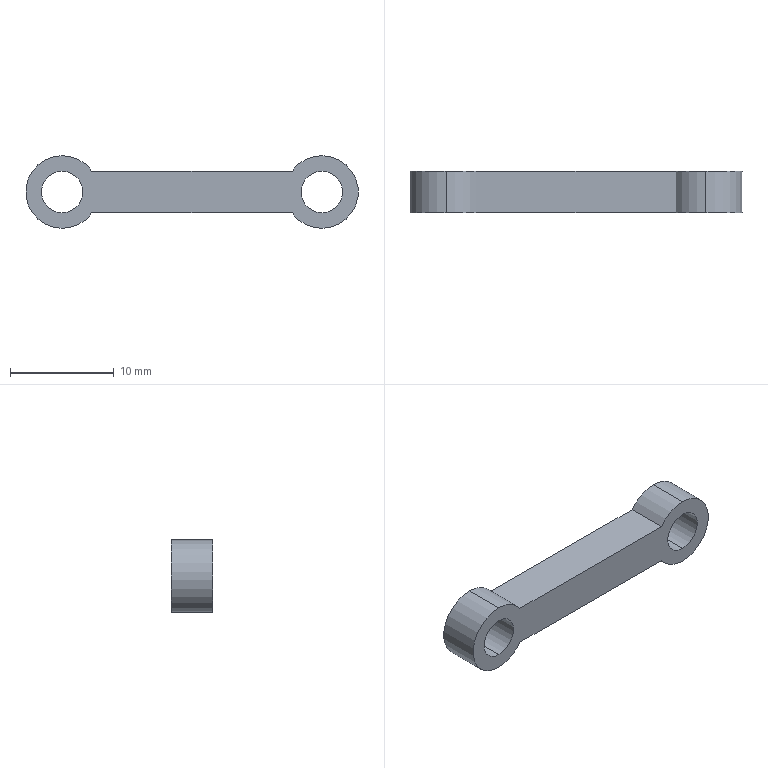Part | SolidWorks | features Extrusion 1, Scale 1 | 1 solid | 14 faces | box 32 x 4 x 7 mm | volume 501.781 mm3 | cylinder 10 | plane 4 | commonest cylinder face diameters 7 x6 4 x4
STEP:
#1=CARTESIAN_POINT('',(25.,4.,-2.));
#2=VERTEX_POINT('',#1);
#3=CARTESIAN_POINT('',(25.,4.,2.));
#4=VERTEX_POINT('',#3);
#5=CARTESIAN_POINT('',(25.,4.,0.));
#6=DIRECTION('',(0.,1.,0.));
#7=DIRECTION('',(0.,0.,1.));
#8=AXIS2_PLACEMENT_3D('',#5,#6,#7);
#9=CIRCLE('',#8,2.);
#10=EDGE_CURVE('',#2,#4,#9,.T.);
#11=ORIENTED_EDGE('',*,*,#10,.T.);
#12=CARTESIAN_POINT('',(25.,0.,2.));
#13=VERTEX_POINT('',#12);
#14=CARTESIAN_POINT('',(25.,4.,2.));
#15=DIRECTION('',(0.,-1.,0.));
#16=VECTOR('',#15,1000.);
#17=LINE('',#14,#16);
#18=EDGE_CURVE('',#4,#13,#17,.T.);
#19=ORIENTED_EDGE('',*,*,#18,.T.);
#20=CARTESIAN_POINT('',(25.,0.,-2.));
#21=VERTEX_POINT('',#20);
#22=CARTESIAN_POINT('',(25.,0.,0.));
#23=DIRECTION('',(0.,1.,0.));
#24=DIRECTION('',(0.,0.,1.));
#25=AXIS2_PLACEMENT_3D('',#22,#23,#24);
#26=CIRCLE('',#25,2.);
#27=EDGE_CURVE('',#21,#13,#26,.T.);
#28=ORIENTED_EDGE('',*,*,#27,.F.);
#29=CARTESIAN_POINT('',(25.,4.,-2.));
#30=DIRECTION('',(0.,-1.,0.));
#31=VECTOR('',#30,1000.);
#32=LINE('',#29,#31);
#33=EDGE_CURVE('',#2,#21,#32,.T.);
#34=ORIENTED_EDGE('',*,*,#33,.F.);
#35=EDGE_LOOP('',(#11,#19,#28,#34));
#36=FACE_OUTER_BOUND('',#35,.T.);
#37=CARTESIAN_POINT('',(25.,4.,0.));
#38=DIRECTION('',(0.,-1.,0.));
#39=DIRECTION('',(0.,0.,-1.));
#40=AXIS2_PLACEMENT_3D('',#37,#38,#39);
#41=CYLINDRICAL_SURFACE('',#40,2.);
#42=ADVANCED_FACE('',(#36),#41,.F.);
#43=CARTESIAN_POINT('',(0.,4.,-2.));
#44=VERTEX_POINT('',#43);
#45=CARTESIAN_POINT('',(0.,4.,2.));
#46=VERTEX_POINT('',#45);
#47=CARTESIAN_POINT('',(0.,4.,0.));
#48=DIRECTION('',(0.,1.,0.));
#49=DIRECTION('',(0.,0.,1.));
#50=AXIS2_PLACEMENT_3D('',#47,#48,#49);
#51=CIRCLE('',#50,2.);
#52=EDGE_CURVE('',#44,#46,#51,.T.);
#53=ORIENTED_EDGE('',*,*,#52,.T.);
#54=CARTESIAN_POINT('',(0.,0.,2.));
#55=VERTEX_POINT('',#54);
#56=CARTESIAN_POINT('',(0.,4.,2.));
#57=DIRECTION('',(0.,-1.,0.));
#58=VECTOR('',#57,1000.);
#59=LINE('',#56,#58);
#60=EDGE_CURVE('',#46,#55,#59,.T.);
#61=ORIENTED_EDGE('',*,*,#60,.T.);
#62=CARTESIAN_POINT('',(0.,0.,-2.));
#63=VERTEX_POINT('',#62);
#64=CARTESIAN_POINT('',(0.,0.,0.));
#65=DIRECTION('',(0.,1.,0.));
#66=DIRECTION('',(0.,0.,1.));
#67=AXIS2_PLACEMENT_3D('',#64,#65,#66);
#68=CIRCLE('',#67,2.);
#69=EDGE_CURVE('',#63,#55,#68,.T.);
#70=ORIENTED_EDGE('',*,*,#69,.F.);
#71=CARTESIAN_POINT('',(0.,4.,-2.));
#72=DIRECTION('',(0.,-1.,0.));
#73=VECTOR('',#72,1000.);
#74=LINE('',#71,#73);
#75=EDGE_CURVE('',#44,#63,#74,.T.);
#76=ORIENTED_EDGE('',*,*,#75,.F.);
#77=EDGE_LOOP('',(#53,#61,#70,#76));
#78=FACE_OUTER_BOUND('',#77,.T.);
#79=CARTESIAN_POINT('',(0.,4.,0.));
#80=DIRECTION('',(0.,-1.,0.));
#81=DIRECTION('',(0.,0.,-1.));
#82=AXIS2_PLACEMENT_3D('',#79,#80,#81);
#83=CYLINDRICAL_SURFACE('',#82,2.);
#84=ADVANCED_FACE('',(#78),#83,.F.);
#85=CARTESIAN_POINT('',(25.,4.,3.5));
#86=VERTEX_POINT('',#85);
#87=CARTESIAN_POINT('',(25.,4.,-3.5));
#88=VERTEX_POINT('',#87);
#89=CARTESIAN_POINT('',(25.,4.,0.));
#90=DIRECTION('',(0.,1.,0.));
#91=DIRECTION('',(0.,0.,1.));
#92=AXIS2_PLACEMENT_3D('',#89,#90,#91);
#93=CIRCLE('',#92,3.5);
#94=EDGE_CURVE('',#86,#88,#93,.T.);
#95=ORIENTED_EDGE('',*,*,#94,.F.);
#96=CARTESIAN_POINT('',(25.,0.,3.5));
#97=VERTEX_POINT('',#96);
#98=CARTESIAN_POINT('',(25.,4.,3.5));
#99=DIRECTION('',(0.,-1.,0.));
#100=VECTOR('',#99,1000.);
#101=LINE('',#98,#100);
#102=EDGE_CURVE('',#86,#97,#101,.T.);
#103=ORIENTED_EDGE('',*,*,#102,.T.);
#104=CARTESIAN_POINT('',(25.,0.,-3.5));
#105=VERTEX_POINT('',#104);
#106=CARTESIAN_POINT('',(25.,0.,0.));
#107=DIRECTION('',(0.,1.,0.));
#108=DIRECTION('',(0.,0.,1.));
#109=AXIS2_PLACEMENT_3D('',#106,#107,#108);
#110=CIRCLE('',#109,3.5);
#111=EDGE_CURVE('',#97,#105,#110,.T.);
#112=ORIENTED_EDGE('',*,*,#111,.T.);
#113=CARTESIAN_POINT('',(25.,4.,-3.5));
#114=DIRECTION('',(0.,-1.,0.));
#115=VECTOR('',#114,1000.);
#116=LINE('',#113,#115);
#117=EDGE_CURVE('',#88,#105,#116,.T.);
#118=ORIENTED_EDGE('',*,*,#117,.F.);
#119=EDGE_LOOP('',(#95,#103,#112,#118));
#120=FACE_OUTER_BOUND('',#119,.T.);
#121=CARTESIAN_POINT('',(25.,4.,0.));
#122=DIRECTION('',(0.,-1.,0.));
#123=DIRECTION('',(0.,0.,-1.));
#124=AXIS2_PLACEMENT_3D('',#121,#122,#123);
#125=CYLINDRICAL_SURFACE('',#124,3.5);
#126=ADVANCED_FACE('',(#120),#125,.T.);
#127=CARTESIAN_POINT('',(22.128,4.,-2.));
#128=VERTEX_POINT('',#127);
#129=CARTESIAN_POINT('',(25.,4.,0.));
#130=DIRECTION('',(0.,1.,0.));
#131=DIRECTION('',(0.,0.,1.));
#132=AXIS2_PLACEMENT_3D('',#129,#130,#131);
#133=CIRCLE('',#132,3.5);
#134=EDGE_CURVE('',#88,#128,#133,.T.);
#135=ORIENTED_EDGE('',*,*,#134,.F.);
#136=ORIENTED_EDGE('',*,*,#117,.T.);
#137=CARTESIAN_POINT('',(22.128,0.,-2.));
#138=VERTEX_POINT('',#137);
#139=CARTESIAN_POINT('',(25.,0.,0.));
#140=DIRECTION('',(0.,1.,0.));
#141=DIRECTION('',(0.,0.,1.));
#142=AXIS2_PLACEMENT_3D('',#139,#140,#141);
#143=CIRCLE('',#142,3.5);
#144=EDGE_CURVE('',#105,#138,#143,.T.);
#145=ORIENTED_EDGE('',*,*,#144,.T.);
#146=CARTESIAN_POINT('',(22.128,4.,-2.));
#147=DIRECTION('',(0.,-1.,0.));
#148=VECTOR('',#147,1000.);
#149=LINE('',#146,#148);
#150=EDGE_CURVE('',#128,#138,#149,.T.);
#151=ORIENTED_EDGE('',*,*,#150,.F.);
#152=EDGE_LOOP('',(#135,#136,#145,#151));
#153=FACE_OUTER_BOUND('',#152,.T.);
#154=CARTESIAN_POINT('',(25.,4.,0.));
#155=DIRECTION('',(0.,-1.,0.));
#156=DIRECTION('',(0.,0.,-1.));
#157=AXIS2_PLACEMENT_3D('',#154,#155,#156);
#158=CYLINDRICAL_SURFACE('',#157,3.5);
#159=ADVANCED_FACE('',(#153),#158,.T.);
#160=CARTESIAN_POINT('',(0.,4.,3.5));
#161=VERTEX_POINT('',#160);
#162=CARTESIAN_POINT('',(2.872,4.,2.));
#163=VERTEX_POINT('',#162);
#164=CARTESIAN_POINT('',(0.,4.,0.));
#165=DIRECTION('',(0.,1.,0.));
#166=DIRECTION('',(0.,0.,1.));
#167=AXIS2_PLACEMENT_3D('',#164,#165,#166);
#168=CIRCLE('',#167,3.5);
#169=EDGE_CURVE('',#161,#163,#168,.T.);
#170=ORIENTED_EDGE('',*,*,#169,.F.);
#171=CARTESIAN_POINT('',(0.,0.,3.5));
#172=VERTEX_POINT('',#171);
#173=CARTESIAN_POINT('',(0.,4.,3.5));
#174=DIRECTION('',(0.,-1.,0.));
#175=VECTOR('',#174,1000.);
#176=LINE('',#173,#175);
#177=EDGE_CURVE('',#161,#172,#176,.T.);
#178=ORIENTED_EDGE('',*,*,#177,.T.);
#179=CARTESIAN_POINT('',(2.872,0.,2.));
#180=VERTEX_POINT('',#179);
#181=CARTESIAN_POINT('',(0.,0.,0.));
#182=DIRECTION('',(0.,1.,0.));
#183=DIRECTION('',(0.,0.,1.));
#184=AXIS2_PLACEMENT_3D('',#181,#182,#183);
#185=CIRCLE('',#184,3.5);
#186=EDGE_CURVE('',#172,#180,#185,.T.);
#187=ORIENTED_EDGE('',*,*,#186,.T.);
#188=CARTESIAN_POINT('',(2.872,4.,2.));
#189=DIRECTION('',(0.,-1.,0.));
#190=VECTOR('',#189,1000.);
#191=LINE('',#188,#190);
#192=EDGE_CURVE('',#163,#180,#191,.T.);
#193=ORIENTED_EDGE('',*,*,#192,.F.);
#194=EDGE_LOOP('',(#170,#178,#187,#193));
#195=FACE_OUTER_BOUND('',#194,.T.);
#196=CARTESIAN_POINT('',(0.,4.,0.));
#197=DIRECTION('',(0.,-1.,0.));
#198=DIRECTION('',(0.,0.,-1.));
#199=AXIS2_PLACEMENT_3D('',#196,#197,#198);
#200=CYLINDRICAL_SURFACE('',#199,3.5);
#201=ADVANCED_FACE('',(#195),#200,.T.);
#202=ORIENTED_EDGE('',*,*,#177,.F.);
#203=CARTESIAN_POINT('',(0.,4.,-3.5));
#204=VERTEX_POINT('',#203);
#205=CARTESIAN_POINT('',(0.,4.,0.));
#206=DIRECTION('',(0.,1.,0.));
#207=DIRECTION('',(0.,0.,1.));
#208=AXIS2_PLACEMENT_3D('',#205,#206,#207);
#209=CIRCLE('',#208,3.5);
#210=EDGE_CURVE('',#204,#161,#209,.T.);
#211=ORIENTED_EDGE('',*,*,#210,.F.);
#212=CARTESIAN_POINT('',(0.,0.,-3.5));
#213=VERTEX_POINT('',#212);
#214=CARTESIAN_POINT('',(0.,4.,-3.5));
#215=DIRECTION('',(0.,-1.,0.));
#216=VECTOR('',#215,1000.);
#217=LINE('',#214,#216);
#218=EDGE_CURVE('',#204,#213,#217,.T.);
#219=ORIENTED_EDGE('',*,*,#218,.T.);
#220=CARTESIAN_POINT('',(0.,0.,0.));
#221=DIRECTION('',(0.,1.,0.));
#222=DIRECTION('',(0.,0.,1.));
#223=AXIS2_PLACEMENT_3D('',#220,#221,#222);
#224=CIRCLE('',#223,3.5);
#225=EDGE_CURVE('',#213,#172,#224,.T.);
#226=ORIENTED_EDGE('',*,*,#225,.T.);
#227=EDGE_LOOP('',(#202,#211,#219,#226));
#228=FACE_OUTER_BOUND('',#227,.T.);
#229=CARTESIAN_POINT('',(0.,4.,0.));
#230=DIRECTION('',(0.,-1.,0.));
#231=DIRECTION('',(0.,0.,-1.));
#232=AXIS2_PLACEMENT_3D('',#229,#230,#231);
#233=CYLINDRICAL_SURFACE('',#232,3.5);
#234=ADVANCED_FACE('',(#228),#233,.T.);
#235=ORIENTED_EDGE('',*,*,#52,.F.);
#236=CARTESIAN_POINT('',(0.,4.,0.));
#237=DIRECTION('',(0.,1.,0.));
#238=DIRECTION('',(0.,0.,1.));
#239=AXIS2_PLACEMENT_3D('',#236,#237,#238);
#240=CIRCLE('',#239,2.);
#241=EDGE_CURVE('',#46,#44,#240,.T.);
#242=ORIENTED_EDGE('',*,*,#241,.F.);
#243=EDGE_LOOP('',(#235,#242));
#244=FACE_BOUND('',#243,.T.);
#245=CARTESIAN_POINT('',(2.872,4.,-2.));
#246=VERTEX_POINT('',#245);
#247=CARTESIAN_POINT('',(0.,4.,0.));
#248=DIRECTION('',(0.,1.,0.));
#249=DIRECTION('',(0.,0.,1.));
#250=AXIS2_PLACEMENT_3D('',#247,#248,#249);
#251=CIRCLE('',#250,3.5);
#252=EDGE_CURVE('',#246,#204,#251,.T.);
#253=ORIENTED_EDGE('',*,*,#252,.T.);
#254=ORIENTED_EDGE('',*,*,#210,.T.);
#255=ORIENTED_EDGE('',*,*,#169,.T.);
#256=CARTESIAN_POINT('',(22.128,4.,2.));
#257=VERTEX_POINT('',#256);
#258=CARTESIAN_POINT('',(2.872,4.,2.));
#259=DIRECTION('',(1.,0.,0.));
#260=VECTOR('',#259,1000.);
#261=LINE('',#258,#260);
#262=EDGE_CURVE('',#163,#257,#261,.T.);
#263=ORIENTED_EDGE('',*,*,#262,.T.);
#264=CARTESIAN_POINT('',(25.,4.,0.));
#265=DIRECTION('',(0.,1.,0.));
#266=DIRECTION('',(0.,0.,1.));
#267=AXIS2_PLACEMENT_3D('',#264,#265,#266);
#268=CIRCLE('',#267,3.5);
#269=EDGE_CURVE('',#257,#86,#268,.T.);
#270=ORIENTED_EDGE('',*,*,#269,.T.);
#271=ORIENTED_EDGE('',*,*,#94,.T.);
#272=ORIENTED_EDGE('',*,*,#134,.T.);
#273=CARTESIAN_POINT('',(2.872,4.,-2.));
#274=DIRECTION('',(-1.,0.,0.));
#275=VECTOR('',#274,1000.);
#276=LINE('',#273,#275);
#277=EDGE_CURVE('',#128,#246,#276,.T.);
#278=ORIENTED_EDGE('',*,*,#277,.T.);
#279=EDGE_LOOP('',(#253,#254,#255,#263,#270,#271,#272,#278));
#280=FACE_OUTER_BOUND('',#279,.T.);
#281=ORIENTED_EDGE('',*,*,#10,.F.);
#282=CARTESIAN_POINT('',(25.,4.,0.));
#283=DIRECTION('',(0.,1.,0.));
#284=DIRECTION('',(0.,0.,1.));
#285=AXIS2_PLACEMENT_3D('',#282,#283,#284);
#286=CIRCLE('',#285,2.);
#287=EDGE_CURVE('',#4,#2,#286,.T.);
#288=ORIENTED_EDGE('',*,*,#287,.F.);
#289=EDGE_LOOP('',(#281,#288));
#290=FACE_BOUND('',#289,.T.);
#291=CARTESIAN_POINT('',(0.,4.,0.));
#292=DIRECTION('',(0.,1.,0.));
#293=DIRECTION('',(0.,0.,1.));
#294=AXIS2_PLACEMENT_3D('',#291,#292,#293);
#295=PLANE('',#294);
#296=ADVANCED_FACE('',(#244,#280,#290),#295,.T.);
#297=CARTESIAN_POINT('',(2.872,0.,-2.));
#298=VERTEX_POINT('',#297);
#299=CARTESIAN_POINT('',(0.,0.,0.));
#300=DIRECTION('',(0.,1.,0.));
#301=DIRECTION('',(0.,0.,1.));
#302=AXIS2_PLACEMENT_3D('',#299,#300,#301);
#303=CIRCLE('',#302,3.5);
#304=EDGE_CURVE('',#298,#213,#303,.T.);
#305=ORIENTED_EDGE('',*,*,#304,.F.);
#306=CARTESIAN_POINT('',(2.872,0.,-2.));
#307=DIRECTION('',(-1.,0.,0.));
#308=VECTOR('',#307,1000.);
#309=LINE('',#306,#308);
#310=EDGE_CURVE('',#138,#298,#309,.T.);
#311=ORIENTED_EDGE('',*,*,#310,.F.);
#312=ORIENTED_EDGE('',*,*,#144,.F.);
#313=ORIENTED_EDGE('',*,*,#111,.F.);
#314=CARTESIAN_POINT('',(22.128,0.,2.));
#315=VERTEX_POINT('',#314);
#316=CARTESIAN_POINT('',(25.,0.,0.));
#317=DIRECTION('',(0.,1.,0.));
#318=DIRECTION('',(0.,0.,1.));
#319=AXIS2_PLACEMENT_3D('',#316,#317,#318);
#320=CIRCLE('',#319,3.5);
#321=EDGE_CURVE('',#315,#97,#320,.T.);
#322=ORIENTED_EDGE('',*,*,#321,.F.);
#323=CARTESIAN_POINT('',(2.872,0.,2.));
#324=DIRECTION('',(1.,0.,0.));
#325=VECTOR('',#324,1000.);
#326=LINE('',#323,#325);
#327=EDGE_CURVE('',#180,#315,#326,.T.);
#328=ORIENTED_EDGE('',*,*,#327,.F.);
#329=ORIENTED_EDGE('',*,*,#186,.F.);
#330=ORIENTED_EDGE('',*,*,#225,.F.);
#331=EDGE_LOOP('',(#305,#311,#312,#313,#322,#328,#329,#330));
#332=FACE_OUTER_BOUND('',#331,.T.);
#333=ORIENTED_EDGE('',*,*,#69,.T.);
#334=CARTESIAN_POINT('',(0.,0.,0.));
#335=DIRECTION('',(0.,1.,0.));
#336=DIRECTION('',(0.,0.,1.));
#337=AXIS2_PLACEMENT_3D('',#334,#335,#336);
#338=CIRCLE('',#337,2.);
#339=EDGE_CURVE('',#55,#63,#338,.T.);
#340=ORIENTED_EDGE('',*,*,#339,.T.);
#341=EDGE_LOOP('',(#333,#340));
#342=FACE_BOUND('',#341,.T.);
#343=ORIENTED_EDGE('',*,*,#27,.T.);
#344=CARTESIAN_POINT('',(25.,0.,0.));
#345=DIRECTION('',(0.,1.,0.));
#346=DIRECTION('',(0.,0.,1.));
#347=AXIS2_PLACEMENT_3D('',#344,#345,#346);
#348=CIRCLE('',#347,2.);
#349=EDGE_CURVE('',#13,#21,#348,.T.);
#350=ORIENTED_EDGE('',*,*,#349,.T.);
#351=EDGE_LOOP('',(#343,#350));
#352=FACE_BOUND('',#351,.T.);
#353=CARTESIAN_POINT('',(0.,0.,0.));
#354=DIRECTION('',(0.,1.,0.));
#355=DIRECTION('',(0.,0.,1.));
#356=AXIS2_PLACEMENT_3D('',#353,#354,#355);
#357=PLANE('',#356);
#358=ADVANCED_FACE('',(#332,#342,#352),#357,.F.);
#359=ORIENTED_EDGE('',*,*,#218,.F.);
#360=ORIENTED_EDGE('',*,*,#252,.F.);
#361=CARTESIAN_POINT('',(2.872,4.,-2.));
#362=DIRECTION('',(0.,-1.,0.));
#363=VECTOR('',#362,1000.);
#364=LINE('',#361,#363);
#365=EDGE_CURVE('',#246,#298,#364,.T.);
#366=ORIENTED_EDGE('',*,*,#365,.T.);
#367=ORIENTED_EDGE('',*,*,#304,.T.);
#368=EDGE_LOOP('',(#359,#360,#366,#367));
#369=FACE_OUTER_BOUND('',#368,.T.);
#370=CARTESIAN_POINT('',(0.,4.,0.));
#371=DIRECTION('',(0.,-1.,0.));
#372=DIRECTION('',(0.,0.,-1.));
#373=AXIS2_PLACEMENT_3D('',#370,#371,#372);
#374=CYLINDRICAL_SURFACE('',#373,3.5);
#375=ADVANCED_FACE('',(#369),#374,.T.);
#376=ORIENTED_EDGE('',*,*,#327,.T.);
#377=CARTESIAN_POINT('',(22.128,4.,2.));
#378=DIRECTION('',(0.,-1.,0.));
#379=VECTOR('',#378,1000.);
#380=LINE('',#377,#379);
#381=EDGE_CURVE('',#257,#315,#380,.T.);
#382=ORIENTED_EDGE('',*,*,#381,.F.);
#383=ORIENTED_EDGE('',*,*,#262,.F.);
#384=ORIENTED_EDGE('',*,*,#192,.T.);
#385=EDGE_LOOP('',(#376,#382,#383,#384));
#386=FACE_OUTER_BOUND('',#385,.T.);
#387=CARTESIAN_POINT('',(2.872,4.,2.));
#388=DIRECTION('',(0.,0.,-1.));
#389=DIRECTION('',(-1.,0.,0.));
#390=AXIS2_PLACEMENT_3D('',#387,#388,#389);
#391=PLANE('',#390);
#392=ADVANCED_FACE('',(#386),#391,.F.);
#393=ORIENTED_EDGE('',*,*,#102,.F.);
#394=ORIENTED_EDGE('',*,*,#269,.F.);
#395=ORIENTED_EDGE('',*,*,#381,.T.);
#396=ORIENTED_EDGE('',*,*,#321,.T.);
#397=EDGE_LOOP('',(#393,#394,#395,#396));
#398=FACE_OUTER_BOUND('',#397,.T.);
#399=CARTESIAN_POINT('',(25.,4.,0.));
#400=DIRECTION('',(0.,-1.,0.));
#401=DIRECTION('',(0.,0.,-1.));
#402=AXIS2_PLACEMENT_3D('',#399,#400,#401);
#403=CYLINDRICAL_SURFACE('',#402,3.5);
#404=ADVANCED_FACE('',(#398),#403,.T.);
#405=ORIENTED_EDGE('',*,*,#310,.T.);
#406=ORIENTED_EDGE('',*,*,#365,.F.);
#407=ORIENTED_EDGE('',*,*,#277,.F.);
#408=ORIENTED_EDGE('',*,*,#150,.T.);
#409=EDGE_LOOP('',(#405,#406,#407,#408));
#410=FACE_OUTER_BOUND('',#409,.T.);
#411=CARTESIAN_POINT('',(2.872,4.,-2.));
#412=DIRECTION('',(0.,0.,1.));
#413=DIRECTION('',(1.,0.,0.));
#414=AXIS2_PLACEMENT_3D('',#411,#412,#413);
#415=PLANE('',#414);
#416=ADVANCED_FACE('',(#410),#415,.F.);
#417=ORIENTED_EDGE('',*,*,#60,.F.);
#418=ORIENTED_EDGE('',*,*,#241,.T.);
#419=ORIENTED_EDGE('',*,*,#75,.T.);
#420=ORIENTED_EDGE('',*,*,#339,.F.);
#421=EDGE_LOOP('',(#417,#418,#419,#420));
#422=FACE_OUTER_BOUND('',#421,.T.);
#423=CARTESIAN_POINT('',(0.,4.,0.));
#424=DIRECTION('',(0.,-1.,0.));
#425=DIRECTION('',(0.,0.,-1.));
#426=AXIS2_PLACEMENT_3D('',#423,#424,#425);
#427=CYLINDRICAL_SURFACE('',#426,2.);
#428=ADVANCED_FACE('',(#422),#427,.F.);
#429=ORIENTED_EDGE('',*,*,#18,.F.);
#430=ORIENTED_EDGE('',*,*,#287,.T.);
#431=ORIENTED_EDGE('',*,*,#33,.T.);
#432=ORIENTED_EDGE('',*,*,#349,.F.);
#433=EDGE_LOOP('',(#429,#430,#431,#432));
#434=FACE_OUTER_BOUND('',#433,.T.);
#435=CARTESIAN_POINT('',(25.,4.,0.));
#436=DIRECTION('',(0.,-1.,0.));
#437=DIRECTION('',(0.,0.,-1.));
#438=AXIS2_PLACEMENT_3D('',#435,#436,#437);
#439=CYLINDRICAL_SURFACE('',#438,2.);
#440=ADVANCED_FACE('',(#434),#439,.F.);
#441=CLOSED_SHELL('',(#42,#84,#126,#159,#201,#234,#296,#358,#375,#392,#404,#416,#428,#440));
#442=MANIFOLD_SOLID_BREP('',#441);
#443=CARTESIAN_POINT('',(0.,0.,0.));
#444=DIRECTION('',(0.,0.,1.));
#445=DIRECTION('',(1.,0.,0.));
#446=AXIS2_PLACEMENT_3D('',#443,#444,#445);
#447=(LENGTH_UNIT()NAMED_UNIT(*)SI_UNIT(.MILLI.,.METRE.));
#448=UNCERTAINTY_MEASURE_WITH_UNIT(LENGTH_MEASURE(0.00001),#447,'','');
#449=(NAMED_UNIT(*)PLANE_ANGLE_UNIT()SI_UNIT($,.RADIAN.));
#450=(NAMED_UNIT(*)SI_UNIT($,.STERADIAN.)SOLID_ANGLE_UNIT());
#451=(GEOMETRIC_REPRESENTATION_CONTEXT(3)GLOBAL_UNCERTAINTY_ASSIGNED_CONTEXT((#448))GLOBAL_UNIT_ASSIGNED_CONTEXT((#447,#449,#450))REPRESENTATION_CONTEXT('',''));
#452=ADVANCED_BREP_SHAPE_REPRESENTATION('',(#442,#446),#451);